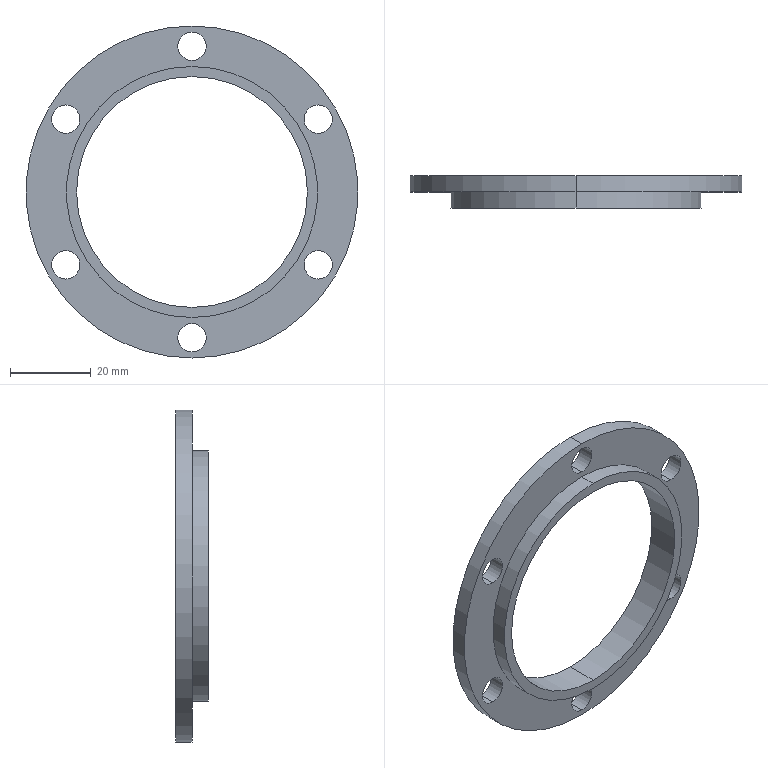Part | SolidWorks | features HoleWzd 2, ICE 1, Revolution 1 | 1 solid | 21 faces | box 82 x 8 x 82 mm | volume 11863 mm3 | cylinder 18 | plane 3 | commonest cylinder face diameters 7 x12 57 x2 62 x2 82 x2
STEP:
#1=CARTESIAN_POINT('',(-1069.592,74.472,129.));
#2=VERTEX_POINT('',#1);
#3=CARTESIAN_POINT('',(-1069.592,74.472,122.));
#4=VERTEX_POINT('',#3);
#5=CARTESIAN_POINT('',(-1069.592,74.472,125.5));
#6=DIRECTION('',(0.,-1.,0.));
#7=DIRECTION('',(0.,0.,-1.));
#8=AXIS2_PLACEMENT_3D('',#5,#6,#7);
#9=CIRCLE('',#8,3.5);
#10=EDGE_CURVE('',#2,#4,#9,.T.);
#11=ORIENTED_EDGE('',*,*,#10,.F.);
#12=CARTESIAN_POINT('',(-1069.592,70.472,129.));
#13=VERTEX_POINT('',#12);
#14=CARTESIAN_POINT('',(-1069.592,70.472,129.));
#15=DIRECTION('',(0.,-1.,0.));
#16=VECTOR('',#15,1000.);
#17=LINE('',#14,#16);
#18=EDGE_CURVE('',#2,#13,#17,.T.);
#19=ORIENTED_EDGE('',*,*,#18,.T.);
#20=CARTESIAN_POINT('',(-1069.592,70.472,122.));
#21=VERTEX_POINT('',#20);
#22=CARTESIAN_POINT('',(-1069.592,70.472,125.5));
#23=DIRECTION('',(0.,-1.,0.));
#24=DIRECTION('',(0.,0.,-1.));
#25=AXIS2_PLACEMENT_3D('',#22,#23,#24);
#26=CIRCLE('',#25,3.5);
#27=EDGE_CURVE('',#13,#21,#26,.T.);
#28=ORIENTED_EDGE('',*,*,#27,.T.);
#29=CARTESIAN_POINT('',(-1069.592,70.472,122.));
#30=DIRECTION('',(0.,-1.,0.));
#31=VECTOR('',#30,1000.);
#32=LINE('',#29,#31);
#33=EDGE_CURVE('',#4,#21,#32,.T.);
#34=ORIENTED_EDGE('',*,*,#33,.F.);
#35=EDGE_LOOP('',(#11,#19,#28,#34));
#36=FACE_OUTER_BOUND('',#35,.T.);
#37=CARTESIAN_POINT('',(-1069.592,70.472,125.5));
#38=DIRECTION('',(0.,-1.,0.));
#39=DIRECTION('',(0.,0.,-1.));
#40=AXIS2_PLACEMENT_3D('',#37,#38,#39);
#41=CYLINDRICAL_SURFACE('',#40,3.5);
#42=ADVANCED_FACE('',(#36),#41,.F.);
#43=CARTESIAN_POINT('',(-1100.769,74.472,111.));
#44=VERTEX_POINT('',#43);
#45=CARTESIAN_POINT('',(-1100.769,74.472,104.));
#46=VERTEX_POINT('',#45);
#47=CARTESIAN_POINT('',(-1100.769,74.472,107.5));
#48=DIRECTION('',(0.,-1.,0.));
#49=DIRECTION('',(0.,0.,-1.));
#50=AXIS2_PLACEMENT_3D('',#47,#48,#49);
#51=CIRCLE('',#50,3.5);
#52=EDGE_CURVE('',#44,#46,#51,.T.);
#53=ORIENTED_EDGE('',*,*,#52,.F.);
#54=CARTESIAN_POINT('',(-1100.769,70.472,111.));
#55=VERTEX_POINT('',#54);
#56=CARTESIAN_POINT('',(-1100.769,70.472,111.));
#57=DIRECTION('',(0.,-1.,0.));
#58=VECTOR('',#57,1000.);
#59=LINE('',#56,#58);
#60=EDGE_CURVE('',#44,#55,#59,.T.);
#61=ORIENTED_EDGE('',*,*,#60,.T.);
#62=CARTESIAN_POINT('',(-1100.769,70.472,104.));
#63=VERTEX_POINT('',#62);
#64=CARTESIAN_POINT('',(-1100.769,70.472,107.5));
#65=DIRECTION('',(0.,-1.,0.));
#66=DIRECTION('',(0.,0.,-1.));
#67=AXIS2_PLACEMENT_3D('',#64,#65,#66);
#68=CIRCLE('',#67,3.5);
#69=EDGE_CURVE('',#55,#63,#68,.T.);
#70=ORIENTED_EDGE('',*,*,#69,.T.);
#71=CARTESIAN_POINT('',(-1100.769,70.472,104.));
#72=DIRECTION('',(0.,-1.,0.));
#73=VECTOR('',#72,1000.);
#74=LINE('',#71,#73);
#75=EDGE_CURVE('',#46,#63,#74,.T.);
#76=ORIENTED_EDGE('',*,*,#75,.F.);
#77=EDGE_LOOP('',(#53,#61,#70,#76));
#78=FACE_OUTER_BOUND('',#77,.T.);
#79=CARTESIAN_POINT('',(-1100.769,70.472,107.5));
#80=DIRECTION('',(0.,-1.,0.));
#81=DIRECTION('',(0.,0.,-1.));
#82=AXIS2_PLACEMENT_3D('',#79,#80,#81);
#83=CYLINDRICAL_SURFACE('',#82,3.5);
#84=ADVANCED_FACE('',(#78),#83,.F.);
#85=CARTESIAN_POINT('',(-1100.769,74.472,75.));
#86=VERTEX_POINT('',#85);
#87=CARTESIAN_POINT('',(-1100.769,74.472,68.));
#88=VERTEX_POINT('',#87);
#89=CARTESIAN_POINT('',(-1100.769,74.472,71.5));
#90=DIRECTION('',(0.,-1.,0.));
#91=DIRECTION('',(0.,0.,-1.));
#92=AXIS2_PLACEMENT_3D('',#89,#90,#91);
#93=CIRCLE('',#92,3.5);
#94=EDGE_CURVE('',#86,#88,#93,.T.);
#95=ORIENTED_EDGE('',*,*,#94,.F.);
#96=CARTESIAN_POINT('',(-1100.769,70.472,75.));
#97=VERTEX_POINT('',#96);
#98=CARTESIAN_POINT('',(-1100.769,70.472,75.));
#99=DIRECTION('',(0.,-1.,0.));
#100=VECTOR('',#99,1000.);
#101=LINE('',#98,#100);
#102=EDGE_CURVE('',#86,#97,#101,.T.);
#103=ORIENTED_EDGE('',*,*,#102,.T.);
#104=CARTESIAN_POINT('',(-1100.769,70.472,68.));
#105=VERTEX_POINT('',#104);
#106=CARTESIAN_POINT('',(-1100.769,70.472,71.5));
#107=DIRECTION('',(0.,-1.,0.));
#108=DIRECTION('',(0.,0.,-1.));
#109=AXIS2_PLACEMENT_3D('',#106,#107,#108);
#110=CIRCLE('',#109,3.5);
#111=EDGE_CURVE('',#97,#105,#110,.T.);
#112=ORIENTED_EDGE('',*,*,#111,.T.);
#113=CARTESIAN_POINT('',(-1100.769,70.472,68.));
#114=DIRECTION('',(0.,-1.,0.));
#115=VECTOR('',#114,1000.);
#116=LINE('',#113,#115);
#117=EDGE_CURVE('',#88,#105,#116,.T.);
#118=ORIENTED_EDGE('',*,*,#117,.F.);
#119=EDGE_LOOP('',(#95,#103,#112,#118));
#120=FACE_OUTER_BOUND('',#119,.T.);
#121=CARTESIAN_POINT('',(-1100.769,70.472,71.5));
#122=DIRECTION('',(0.,-1.,0.));
#123=DIRECTION('',(0.,0.,-1.));
#124=AXIS2_PLACEMENT_3D('',#121,#122,#123);
#125=CYLINDRICAL_SURFACE('',#124,3.5);
#126=ADVANCED_FACE('',(#120),#125,.F.);
#127=CARTESIAN_POINT('',(-1069.592,74.472,57.));
#128=VERTEX_POINT('',#127);
#129=CARTESIAN_POINT('',(-1069.592,74.472,50.));
#130=VERTEX_POINT('',#129);
#131=CARTESIAN_POINT('',(-1069.592,74.472,53.5));
#132=DIRECTION('',(0.,-1.,0.));
#133=DIRECTION('',(0.,0.,-1.));
#134=AXIS2_PLACEMENT_3D('',#131,#132,#133);
#135=CIRCLE('',#134,3.5);
#136=EDGE_CURVE('',#128,#130,#135,.T.);
#137=ORIENTED_EDGE('',*,*,#136,.F.);
#138=CARTESIAN_POINT('',(-1069.592,70.472,57.));
#139=VERTEX_POINT('',#138);
#140=CARTESIAN_POINT('',(-1069.592,70.472,57.));
#141=DIRECTION('',(0.,-1.,0.));
#142=VECTOR('',#141,1000.);
#143=LINE('',#140,#142);
#144=EDGE_CURVE('',#128,#139,#143,.T.);
#145=ORIENTED_EDGE('',*,*,#144,.T.);
#146=CARTESIAN_POINT('',(-1069.592,70.472,50.));
#147=VERTEX_POINT('',#146);
#148=CARTESIAN_POINT('',(-1069.592,70.472,53.5));
#149=DIRECTION('',(0.,-1.,0.));
#150=DIRECTION('',(0.,0.,-1.));
#151=AXIS2_PLACEMENT_3D('',#148,#149,#150);
#152=CIRCLE('',#151,3.5);
#153=EDGE_CURVE('',#139,#147,#152,.T.);
#154=ORIENTED_EDGE('',*,*,#153,.T.);
#155=CARTESIAN_POINT('',(-1069.592,70.472,50.));
#156=DIRECTION('',(0.,-1.,0.));
#157=VECTOR('',#156,1000.);
#158=LINE('',#155,#157);
#159=EDGE_CURVE('',#130,#147,#158,.T.);
#160=ORIENTED_EDGE('',*,*,#159,.F.);
#161=EDGE_LOOP('',(#137,#145,#154,#160));
#162=FACE_OUTER_BOUND('',#161,.T.);
#163=CARTESIAN_POINT('',(-1069.592,70.472,53.5));
#164=DIRECTION('',(0.,-1.,0.));
#165=DIRECTION('',(0.,0.,-1.));
#166=AXIS2_PLACEMENT_3D('',#163,#164,#165);
#167=CYLINDRICAL_SURFACE('',#166,3.5);
#168=ADVANCED_FACE('',(#162),#167,.F.);
#169=CARTESIAN_POINT('',(-1038.415,74.472,75.));
#170=VERTEX_POINT('',#169);
#171=CARTESIAN_POINT('',(-1038.415,74.472,68.));
#172=VERTEX_POINT('',#171);
#173=CARTESIAN_POINT('',(-1038.415,74.472,71.5));
#174=DIRECTION('',(0.,-1.,0.));
#175=DIRECTION('',(0.,0.,-1.));
#176=AXIS2_PLACEMENT_3D('',#173,#174,#175);
#177=CIRCLE('',#176,3.5);
#178=EDGE_CURVE('',#170,#172,#177,.T.);
#179=ORIENTED_EDGE('',*,*,#178,.F.);
#180=CARTESIAN_POINT('',(-1038.415,70.472,75.));
#181=VERTEX_POINT('',#180);
#182=CARTESIAN_POINT('',(-1038.415,70.472,75.));
#183=DIRECTION('',(0.,-1.,0.));
#184=VECTOR('',#183,1000.);
#185=LINE('',#182,#184);
#186=EDGE_CURVE('',#170,#181,#185,.T.);
#187=ORIENTED_EDGE('',*,*,#186,.T.);
#188=CARTESIAN_POINT('',(-1038.415,70.472,68.));
#189=VERTEX_POINT('',#188);
#190=CARTESIAN_POINT('',(-1038.415,70.472,71.5));
#191=DIRECTION('',(0.,-1.,0.));
#192=DIRECTION('',(0.,0.,-1.));
#193=AXIS2_PLACEMENT_3D('',#190,#191,#192);
#194=CIRCLE('',#193,3.5);
#195=EDGE_CURVE('',#181,#189,#194,.T.);
#196=ORIENTED_EDGE('',*,*,#195,.T.);
#197=CARTESIAN_POINT('',(-1038.415,70.472,68.));
#198=DIRECTION('',(0.,-1.,0.));
#199=VECTOR('',#198,1000.);
#200=LINE('',#197,#199);
#201=EDGE_CURVE('',#172,#189,#200,.T.);
#202=ORIENTED_EDGE('',*,*,#201,.F.);
#203=EDGE_LOOP('',(#179,#187,#196,#202));
#204=FACE_OUTER_BOUND('',#203,.T.);
#205=CARTESIAN_POINT('',(-1038.415,70.472,71.5));
#206=DIRECTION('',(0.,-1.,0.));
#207=DIRECTION('',(0.,0.,-1.));
#208=AXIS2_PLACEMENT_3D('',#205,#206,#207);
#209=CYLINDRICAL_SURFACE('',#208,3.5);
#210=ADVANCED_FACE('',(#204),#209,.F.);
#211=CARTESIAN_POINT('',(-1038.415,74.472,111.));
#212=VERTEX_POINT('',#211);
#213=CARTESIAN_POINT('',(-1038.415,74.472,104.));
#214=VERTEX_POINT('',#213);
#215=CARTESIAN_POINT('',(-1038.415,74.472,107.5));
#216=DIRECTION('',(0.,-1.,0.));
#217=DIRECTION('',(0.,0.,-1.));
#218=AXIS2_PLACEMENT_3D('',#215,#216,#217);
#219=CIRCLE('',#218,3.5);
#220=EDGE_CURVE('',#212,#214,#219,.T.);
#221=ORIENTED_EDGE('',*,*,#220,.F.);
#222=CARTESIAN_POINT('',(-1038.415,70.472,111.));
#223=VERTEX_POINT('',#222);
#224=CARTESIAN_POINT('',(-1038.415,70.472,111.));
#225=DIRECTION('',(0.,-1.,0.));
#226=VECTOR('',#225,1000.);
#227=LINE('',#224,#226);
#228=EDGE_CURVE('',#212,#223,#227,.T.);
#229=ORIENTED_EDGE('',*,*,#228,.T.);
#230=CARTESIAN_POINT('',(-1038.415,70.472,104.));
#231=VERTEX_POINT('',#230);
#232=CARTESIAN_POINT('',(-1038.415,70.472,107.5));
#233=DIRECTION('',(0.,-1.,0.));
#234=DIRECTION('',(0.,0.,-1.));
#235=AXIS2_PLACEMENT_3D('',#232,#233,#234);
#236=CIRCLE('',#235,3.5);
#237=EDGE_CURVE('',#223,#231,#236,.T.);
#238=ORIENTED_EDGE('',*,*,#237,.T.);
#239=CARTESIAN_POINT('',(-1038.415,70.472,104.));
#240=DIRECTION('',(0.,-1.,0.));
#241=VECTOR('',#240,1000.);
#242=LINE('',#239,#241);
#243=EDGE_CURVE('',#214,#231,#242,.T.);
#244=ORIENTED_EDGE('',*,*,#243,.F.);
#245=EDGE_LOOP('',(#221,#229,#238,#244));
#246=FACE_OUTER_BOUND('',#245,.T.);
#247=CARTESIAN_POINT('',(-1038.415,70.472,107.5));
#248=DIRECTION('',(0.,-1.,0.));
#249=DIRECTION('',(0.,0.,-1.));
#250=AXIS2_PLACEMENT_3D('',#247,#248,#249);
#251=CYLINDRICAL_SURFACE('',#250,3.5);
#252=ADVANCED_FACE('',(#246),#251,.F.);
#253=CARTESIAN_POINT('',(-1069.592,74.472,118.));
#254=VERTEX_POINT('',#253);
#255=CARTESIAN_POINT('',(-1069.592,74.472,61.));
#256=VERTEX_POINT('',#255);
#257=CARTESIAN_POINT('',(-1069.592,74.472,89.5));
#258=DIRECTION('',(0.,-1.,0.));
#259=DIRECTION('',(0.,0.,-1.));
#260=AXIS2_PLACEMENT_3D('',#257,#258,#259);
#261=CIRCLE('',#260,28.5);
#262=EDGE_CURVE('',#254,#256,#261,.T.);
#263=ORIENTED_EDGE('',*,*,#262,.F.);
#264=CARTESIAN_POINT('',(-1069.592,66.472,118.));
#265=VERTEX_POINT('',#264);
#266=CARTESIAN_POINT('',(-1069.592,66.472,118.));
#267=DIRECTION('',(0.,-1.,0.));
#268=VECTOR('',#267,1000.);
#269=LINE('',#266,#268);
#270=EDGE_CURVE('',#254,#265,#269,.T.);
#271=ORIENTED_EDGE('',*,*,#270,.T.);
#272=CARTESIAN_POINT('',(-1069.592,66.472,61.));
#273=VERTEX_POINT('',#272);
#274=CARTESIAN_POINT('',(-1069.592,66.472,89.5));
#275=DIRECTION('',(0.,-1.,0.));
#276=DIRECTION('',(0.,0.,-1.));
#277=AXIS2_PLACEMENT_3D('',#274,#275,#276);
#278=CIRCLE('',#277,28.5);
#279=EDGE_CURVE('',#265,#273,#278,.T.);
#280=ORIENTED_EDGE('',*,*,#279,.T.);
#281=CARTESIAN_POINT('',(-1069.592,66.472,61.));
#282=DIRECTION('',(0.,-1.,0.));
#283=VECTOR('',#282,1000.);
#284=LINE('',#281,#283);
#285=EDGE_CURVE('',#256,#273,#284,.T.);
#286=ORIENTED_EDGE('',*,*,#285,.F.);
#287=EDGE_LOOP('',(#263,#271,#280,#286));
#288=FACE_OUTER_BOUND('',#287,.T.);
#289=CARTESIAN_POINT('',(-1069.592,66.472,89.5));
#290=DIRECTION('',(0.,-1.,0.));
#291=DIRECTION('',(0.,0.,-1.));
#292=AXIS2_PLACEMENT_3D('',#289,#290,#291);
#293=CYLINDRICAL_SURFACE('',#292,28.5);
#294=ADVANCED_FACE('',(#288),#293,.F.);
#295=CARTESIAN_POINT('',(-1069.592,66.472,58.5));
#296=VERTEX_POINT('',#295);
#297=CARTESIAN_POINT('',(-1069.592,66.472,120.5));
#298=VERTEX_POINT('',#297);
#299=CARTESIAN_POINT('',(-1069.592,66.472,89.5));
#300=DIRECTION('',(0.,-1.,0.));
#301=DIRECTION('',(0.,0.,-1.));
#302=AXIS2_PLACEMENT_3D('',#299,#300,#301);
#303=CIRCLE('',#302,31.);
#304=EDGE_CURVE('',#296,#298,#303,.T.);
#305=ORIENTED_EDGE('',*,*,#304,.F.);
#306=CARTESIAN_POINT('',(-1069.592,70.472,58.5));
#307=VERTEX_POINT('',#306);
#308=CARTESIAN_POINT('',(-1069.592,66.472,58.5));
#309=DIRECTION('',(0.,1.,0.));
#310=VECTOR('',#309,1000.);
#311=LINE('',#308,#310);
#312=EDGE_CURVE('',#296,#307,#311,.T.);
#313=ORIENTED_EDGE('',*,*,#312,.T.);
#314=CARTESIAN_POINT('',(-1069.592,70.472,120.5));
#315=VERTEX_POINT('',#314);
#316=CARTESIAN_POINT('',(-1069.592,70.472,89.5));
#317=DIRECTION('',(0.,-1.,0.));
#318=DIRECTION('',(0.,0.,-1.));
#319=AXIS2_PLACEMENT_3D('',#316,#317,#318);
#320=CIRCLE('',#319,31.);
#321=EDGE_CURVE('',#307,#315,#320,.T.);
#322=ORIENTED_EDGE('',*,*,#321,.T.);
#323=CARTESIAN_POINT('',(-1069.592,66.472,120.5));
#324=DIRECTION('',(0.,1.,0.));
#325=VECTOR('',#324,1000.);
#326=LINE('',#323,#325);
#327=EDGE_CURVE('',#298,#315,#326,.T.);
#328=ORIENTED_EDGE('',*,*,#327,.F.);
#329=EDGE_LOOP('',(#305,#313,#322,#328));
#330=FACE_OUTER_BOUND('',#329,.T.);
#331=CARTESIAN_POINT('',(-1069.592,66.472,89.5));
#332=DIRECTION('',(0.,1.,0.));
#333=DIRECTION('',(0.,0.,1.));
#334=AXIS2_PLACEMENT_3D('',#331,#332,#333);
#335=CYLINDRICAL_SURFACE('',#334,31.);
#336=ADVANCED_FACE('',(#330),#335,.T.);
#337=CARTESIAN_POINT('',(-1069.592,74.472,48.5));
#338=VERTEX_POINT('',#337);
#339=CARTESIAN_POINT('',(-1069.592,74.472,130.5));
#340=VERTEX_POINT('',#339);
#341=CARTESIAN_POINT('',(-1069.592,74.472,89.5));
#342=DIRECTION('',(0.,-1.,0.));
#343=DIRECTION('',(0.,0.,-1.));
#344=AXIS2_PLACEMENT_3D('',#341,#342,#343);
#345=CIRCLE('',#344,41.);
#346=EDGE_CURVE('',#338,#340,#345,.T.);
#347=ORIENTED_EDGE('',*,*,#346,.T.);
#348=CARTESIAN_POINT('',(-1069.592,70.472,130.5));
#349=VERTEX_POINT('',#348);
#350=CARTESIAN_POINT('',(-1069.592,74.472,130.5));
#351=DIRECTION('',(0.,-1.,0.));
#352=VECTOR('',#351,1000.);
#353=LINE('',#350,#352);
#354=EDGE_CURVE('',#340,#349,#353,.T.);
#355=ORIENTED_EDGE('',*,*,#354,.T.);
#356=CARTESIAN_POINT('',(-1069.592,70.472,48.5));
#357=VERTEX_POINT('',#356);
#358=CARTESIAN_POINT('',(-1069.592,70.472,89.5));
#359=DIRECTION('',(0.,-1.,0.));
#360=DIRECTION('',(0.,0.,-1.));
#361=AXIS2_PLACEMENT_3D('',#358,#359,#360);
#362=CIRCLE('',#361,41.);
#363=EDGE_CURVE('',#357,#349,#362,.T.);
#364=ORIENTED_EDGE('',*,*,#363,.F.);
#365=CARTESIAN_POINT('',(-1069.592,74.472,48.5));
#366=DIRECTION('',(0.,-1.,0.));
#367=VECTOR('',#366,1000.);
#368=LINE('',#365,#367);
#369=EDGE_CURVE('',#338,#357,#368,.T.);
#370=ORIENTED_EDGE('',*,*,#369,.F.);
#371=EDGE_LOOP('',(#347,#355,#364,#370));
#372=FACE_OUTER_BOUND('',#371,.T.);
#373=CARTESIAN_POINT('',(-1069.592,74.472,89.5));
#374=DIRECTION('',(0.,-1.,0.));
#375=DIRECTION('',(0.,0.,-1.));
#376=AXIS2_PLACEMENT_3D('',#373,#374,#375);
#377=CYLINDRICAL_SURFACE('',#376,41.);
#378=ADVANCED_FACE('',(#372),#377,.T.);
#379=ORIENTED_EDGE('',*,*,#354,.F.);
#380=CARTESIAN_POINT('',(-1069.592,74.472,89.5));
#381=DIRECTION('',(0.,-1.,0.));
#382=DIRECTION('',(0.,0.,-1.));
#383=AXIS2_PLACEMENT_3D('',#380,#381,#382);
#384=CIRCLE('',#383,41.);
#385=EDGE_CURVE('',#340,#338,#384,.T.);
#386=ORIENTED_EDGE('',*,*,#385,.T.);
#387=ORIENTED_EDGE('',*,*,#369,.T.);
#388=CARTESIAN_POINT('',(-1069.592,70.472,89.5));
#389=DIRECTION('',(0.,-1.,0.));
#390=DIRECTION('',(0.,0.,-1.));
#391=AXIS2_PLACEMENT_3D('',#388,#389,#390);
#392=CIRCLE('',#391,41.);
#393=EDGE_CURVE('',#349,#357,#392,.T.);
#394=ORIENTED_EDGE('',*,*,#393,.F.);
#395=EDGE_LOOP('',(#379,#386,#387,#394));
#396=FACE_OUTER_BOUND('',#395,.T.);
#397=CARTESIAN_POINT('',(-1069.592,74.472,89.5));
#398=DIRECTION('',(0.,-1.,0.));
#399=DIRECTION('',(0.,0.,-1.));
#400=AXIS2_PLACEMENT_3D('',#397,#398,#399);
#401=CYLINDRICAL_SURFACE('',#400,41.);
#402=ADVANCED_FACE('',(#396),#401,.T.);
#403=CARTESIAN_POINT('',(-1069.592,74.472,125.5));
#404=DIRECTION('',(0.,-1.,0.));
#405=DIRECTION('',(0.,0.,-1.));
#406=AXIS2_PLACEMENT_3D('',#403,#404,#405);
#407=CIRCLE('',#406,3.5);
#408=EDGE_CURVE('',#4,#2,#407,.T.);
#409=ORIENTED_EDGE('',*,*,#408,.T.);
#410=ORIENTED_EDGE('',*,*,#10,.T.);
#411=EDGE_LOOP('',(#409,#410));
#412=FACE_BOUND('',#411,.T.);
#413=CARTESIAN_POINT('',(-1100.769,74.472,107.5));
#414=DIRECTION('',(0.,-1.,0.));
#415=DIRECTION('',(0.,0.,-1.));
#416=AXIS2_PLACEMENT_3D('',#413,#414,#415);
#417=CIRCLE('',#416,3.5);
#418=EDGE_CURVE('',#46,#44,#417,.T.);
#419=ORIENTED_EDGE('',*,*,#418,.T.);
#420=ORIENTED_EDGE('',*,*,#52,.T.);
#421=EDGE_LOOP('',(#419,#420));
#422=FACE_BOUND('',#421,.T.);
#423=CARTESIAN_POINT('',(-1100.769,74.472,71.5));
#424=DIRECTION('',(0.,-1.,0.));
#425=DIRECTION('',(0.,0.,-1.));
#426=AXIS2_PLACEMENT_3D('',#423,#424,#425);
#427=CIRCLE('',#426,3.5);
#428=EDGE_CURVE('',#88,#86,#427,.T.);
#429=ORIENTED_EDGE('',*,*,#428,.T.);
#430=ORIENTED_EDGE('',*,*,#94,.T.);
#431=EDGE_LOOP('',(#429,#430));
#432=FACE_BOUND('',#431,.T.);
#433=CARTESIAN_POINT('',(-1069.592,74.472,53.5));
#434=DIRECTION('',(0.,-1.,0.));
#435=DIRECTION('',(0.,0.,-1.));
#436=AXIS2_PLACEMENT_3D('',#433,#434,#435);
#437=CIRCLE('',#436,3.5);
#438=EDGE_CURVE('',#130,#128,#437,.T.);
#439=ORIENTED_EDGE('',*,*,#438,.T.);
#440=ORIENTED_EDGE('',*,*,#136,.T.);
#441=EDGE_LOOP('',(#439,#440));
#442=FACE_BOUND('',#441,.T.);
#443=CARTESIAN_POINT('',(-1038.415,74.472,71.5));
#444=DIRECTION('',(0.,-1.,0.));
#445=DIRECTION('',(0.,0.,-1.));
#446=AXIS2_PLACEMENT_3D('',#443,#444,#445);
#447=CIRCLE('',#446,3.5);
#448=EDGE_CURVE('',#172,#170,#447,.T.);
#449=ORIENTED_EDGE('',*,*,#448,.T.);
#450=ORIENTED_EDGE('',*,*,#178,.T.);
#451=EDGE_LOOP('',(#449,#450));
#452=FACE_BOUND('',#451,.T.);
#453=CARTESIAN_POINT('',(-1038.415,74.472,107.5));
#454=DIRECTION('',(0.,-1.,0.));
#455=DIRECTION('',(0.,0.,-1.));
#456=AXIS2_PLACEMENT_3D('',#453,#454,#455);
#457=CIRCLE('',#456,3.5);
#458=EDGE_CURVE('',#214,#212,#457,.T.);
#459=ORIENTED_EDGE('',*,*,#458,.T.);
#460=ORIENTED_EDGE('',*,*,#220,.T.);
#461=EDGE_LOOP('',(#459,#460));
#462=FACE_BOUND('',#461,.T.);
#463=CARTESIAN_POINT('',(-1069.592,74.472,89.5));
#464=DIRECTION('',(0.,-1.,0.));
#465=DIRECTION('',(0.,0.,-1.));
#466=AXIS2_PLACEMENT_3D('',#463,#464,#465);
#467=CIRCLE('',#466,28.5);
#468=EDGE_CURVE('',#256,#254,#467,.T.);
#469=ORIENTED_EDGE('',*,*,#468,.T.);
#470=ORIENTED_EDGE('',*,*,#262,.T.);
#471=EDGE_LOOP('',(#469,#470));
#472=FACE_BOUND('',#471,.T.);
#473=ORIENTED_EDGE('',*,*,#346,.F.);
#474=ORIENTED_EDGE('',*,*,#385,.F.);
#475=EDGE_LOOP('',(#473,#474));
#476=FACE_OUTER_BOUND('',#475,.T.);
#477=CARTESIAN_POINT('',(-1028.592,74.472,89.5));
#478=DIRECTION('',(0.,1.,0.));
#479=DIRECTION('',(0.,0.,1.));
#480=AXIS2_PLACEMENT_3D('',#477,#478,#479);
#481=PLANE('',#480);
#482=ADVANCED_FACE('',(#412,#422,#432,#442,#452,#462,#472,#476),#481,.T.);
#483=CARTESIAN_POINT('',(-1069.592,70.472,125.5));
#484=DIRECTION('',(0.,-1.,0.));
#485=DIRECTION('',(0.,0.,-1.));
#486=AXIS2_PLACEMENT_3D('',#483,#484,#485);
#487=CIRCLE('',#486,3.5);
#488=EDGE_CURVE('',#21,#13,#487,.T.);
#489=ORIENTED_EDGE('',*,*,#488,.F.);
#490=ORIENTED_EDGE('',*,*,#27,.F.);
#491=EDGE_LOOP('',(#489,#490));
#492=FACE_BOUND('',#491,.T.);
#493=CARTESIAN_POINT('',(-1100.769,70.472,107.5));
#494=DIRECTION('',(0.,-1.,0.));
#495=DIRECTION('',(0.,0.,-1.));
#496=AXIS2_PLACEMENT_3D('',#493,#494,#495);
#497=CIRCLE('',#496,3.5);
#498=EDGE_CURVE('',#63,#55,#497,.T.);
#499=ORIENTED_EDGE('',*,*,#498,.F.);
#500=ORIENTED_EDGE('',*,*,#69,.F.);
#501=EDGE_LOOP('',(#499,#500));
#502=FACE_BOUND('',#501,.T.);
#503=CARTESIAN_POINT('',(-1100.769,70.472,71.5));
#504=DIRECTION('',(0.,-1.,0.));
#505=DIRECTION('',(0.,0.,-1.));
#506=AXIS2_PLACEMENT_3D('',#503,#504,#505);
#507=CIRCLE('',#506,3.5);
#508=EDGE_CURVE('',#105,#97,#507,.T.);
#509=ORIENTED_EDGE('',*,*,#508,.F.);
#510=ORIENTED_EDGE('',*,*,#111,.F.);
#511=EDGE_LOOP('',(#509,#510));
#512=FACE_BOUND('',#511,.T.);
#513=CARTESIAN_POINT('',(-1069.592,70.472,53.5));
#514=DIRECTION('',(0.,-1.,0.));
#515=DIRECTION('',(0.,0.,-1.));
#516=AXIS2_PLACEMENT_3D('',#513,#514,#515);
#517=CIRCLE('',#516,3.5);
#518=EDGE_CURVE('',#147,#139,#517,.T.);
#519=ORIENTED_EDGE('',*,*,#518,.F.);
#520=ORIENTED_EDGE('',*,*,#153,.F.);
#521=EDGE_LOOP('',(#519,#520));
#522=FACE_BOUND('',#521,.T.);
#523=CARTESIAN_POINT('',(-1038.415,70.472,71.5));
#524=DIRECTION('',(0.,-1.,0.));
#525=DIRECTION('',(0.,0.,-1.));
#526=AXIS2_PLACEMENT_3D('',#523,#524,#525);
#527=CIRCLE('',#526,3.5);
#528=EDGE_CURVE('',#189,#181,#527,.T.);
#529=ORIENTED_EDGE('',*,*,#528,.F.);
#530=ORIENTED_EDGE('',*,*,#195,.F.);
#531=EDGE_LOOP('',(#529,#530));
#532=FACE_BOUND('',#531,.T.);
#533=CARTESIAN_POINT('',(-1038.415,70.472,107.5));
#534=DIRECTION('',(0.,-1.,0.));
#535=DIRECTION('',(0.,0.,-1.));
#536=AXIS2_PLACEMENT_3D('',#533,#534,#535);
#537=CIRCLE('',#536,3.5);
#538=EDGE_CURVE('',#231,#223,#537,.T.);
#539=ORIENTED_EDGE('',*,*,#538,.F.);
#540=ORIENTED_EDGE('',*,*,#237,.F.);
#541=EDGE_LOOP('',(#539,#540));
#542=FACE_BOUND('',#541,.T.);
#543=CARTESIAN_POINT('',(-1069.592,70.472,89.5));
#544=DIRECTION('',(0.,-1.,0.));
#545=DIRECTION('',(0.,0.,-1.));
#546=AXIS2_PLACEMENT_3D('',#543,#544,#545);
#547=CIRCLE('',#546,31.);
#548=EDGE_CURVE('',#315,#307,#547,.T.);
#549=ORIENTED_EDGE('',*,*,#548,.F.);
#550=ORIENTED_EDGE('',*,*,#321,.F.);
#551=EDGE_LOOP('',(#549,#550));
#552=FACE_BOUND('',#551,.T.);
#553=ORIENTED_EDGE('',*,*,#363,.T.);
#554=ORIENTED_EDGE('',*,*,#393,.T.);
#555=EDGE_LOOP('',(#553,#554));
#556=FACE_OUTER_BOUND('',#555,.T.);
#557=CARTESIAN_POINT('',(-1069.592,70.472,89.5));
#558=DIRECTION('',(0.,-1.,0.));
#559=DIRECTION('',(0.,0.,-1.));
#560=AXIS2_PLACEMENT_3D('',#557,#558,#559);
#561=PLANE('',#560);
#562=ADVANCED_FACE('',(#492,#502,#512,#522,#532,#542,#552,#556),#561,.T.);
#563=ORIENTED_EDGE('',*,*,#312,.F.);
#564=CARTESIAN_POINT('',(-1069.592,66.472,89.5));
#565=DIRECTION('',(0.,-1.,0.));
#566=DIRECTION('',(0.,0.,-1.));
#567=AXIS2_PLACEMENT_3D('',#564,#565,#566);
#568=CIRCLE('',#567,31.);
#569=EDGE_CURVE('',#298,#296,#568,.T.);
#570=ORIENTED_EDGE('',*,*,#569,.F.);
#571=ORIENTED_EDGE('',*,*,#327,.T.);
#572=ORIENTED_EDGE('',*,*,#548,.T.);
#573=EDGE_LOOP('',(#563,#570,#571,#572));
#574=FACE_OUTER_BOUND('',#573,.T.);
#575=CARTESIAN_POINT('',(-1069.592,66.472,89.5));
#576=DIRECTION('',(0.,1.,0.));
#577=DIRECTION('',(0.,0.,1.));
#578=AXIS2_PLACEMENT_3D('',#575,#576,#577);
#579=CYLINDRICAL_SURFACE('',#578,31.);
#580=ADVANCED_FACE('',(#574),#579,.T.);
#581=CARTESIAN_POINT('',(-1069.592,66.472,89.5));
#582=DIRECTION('',(0.,-1.,0.));
#583=DIRECTION('',(0.,0.,-1.));
#584=AXIS2_PLACEMENT_3D('',#581,#582,#583);
#585=CIRCLE('',#584,28.5);
#586=EDGE_CURVE('',#273,#265,#585,.T.);
#587=ORIENTED_EDGE('',*,*,#586,.F.);
#588=ORIENTED_EDGE('',*,*,#279,.F.);
#589=EDGE_LOOP('',(#587,#588));
#590=FACE_BOUND('',#589,.T.);
#591=ORIENTED_EDGE('',*,*,#569,.T.);
#592=ORIENTED_EDGE('',*,*,#304,.T.);
#593=EDGE_LOOP('',(#591,#592));
#594=FACE_OUTER_BOUND('',#593,.T.);
#595=CARTESIAN_POINT('',(-1069.592,66.472,89.5));
#596=DIRECTION('',(0.,-1.,0.));
#597=DIRECTION('',(0.,0.,-1.));
#598=AXIS2_PLACEMENT_3D('',#595,#596,#597);
#599=PLANE('',#598);
#600=ADVANCED_FACE('',(#590,#594),#599,.T.);
#601=ORIENTED_EDGE('',*,*,#270,.F.);
#602=ORIENTED_EDGE('',*,*,#468,.F.);
#603=ORIENTED_EDGE('',*,*,#285,.T.);
#604=ORIENTED_EDGE('',*,*,#586,.T.);
#605=EDGE_LOOP('',(#601,#602,#603,#604));
#606=FACE_OUTER_BOUND('',#605,.T.);
#607=CARTESIAN_POINT('',(-1069.592,66.472,89.5));
#608=DIRECTION('',(0.,-1.,0.));
#609=DIRECTION('',(0.,0.,-1.));
#610=AXIS2_PLACEMENT_3D('',#607,#608,#609);
#611=CYLINDRICAL_SURFACE('',#610,28.5);
#612=ADVANCED_FACE('',(#606),#611,.F.);
#613=ORIENTED_EDGE('',*,*,#228,.F.);
#614=ORIENTED_EDGE('',*,*,#458,.F.);
#615=ORIENTED_EDGE('',*,*,#243,.T.);
#616=ORIENTED_EDGE('',*,*,#538,.T.);
#617=EDGE_LOOP('',(#613,#614,#615,#616));
#618=FACE_OUTER_BOUND('',#617,.T.);
#619=CARTESIAN_POINT('',(-1038.415,70.472,107.5));
#620=DIRECTION('',(0.,-1.,0.));
#621=DIRECTION('',(0.,0.,-1.));
#622=AXIS2_PLACEMENT_3D('',#619,#620,#621);
#623=CYLINDRICAL_SURFACE('',#622,3.5);
#624=ADVANCED_FACE('',(#618),#623,.F.);
#625=ORIENTED_EDGE('',*,*,#186,.F.);
#626=ORIENTED_EDGE('',*,*,#448,.F.);
#627=ORIENTED_EDGE('',*,*,#201,.T.);
#628=ORIENTED_EDGE('',*,*,#528,.T.);
#629=EDGE_LOOP('',(#625,#626,#627,#628));
#630=FACE_OUTER_BOUND('',#629,.T.);
#631=CARTESIAN_POINT('',(-1038.415,70.472,71.5));
#632=DIRECTION('',(0.,-1.,0.));
#633=DIRECTION('',(0.,0.,-1.));
#634=AXIS2_PLACEMENT_3D('',#631,#632,#633);
#635=CYLINDRICAL_SURFACE('',#634,3.5);
#636=ADVANCED_FACE('',(#630),#635,.F.);
#637=ORIENTED_EDGE('',*,*,#144,.F.);
#638=ORIENTED_EDGE('',*,*,#438,.F.);
#639=ORIENTED_EDGE('',*,*,#159,.T.);
#640=ORIENTED_EDGE('',*,*,#518,.T.);
#641=EDGE_LOOP('',(#637,#638,#639,#640));
#642=FACE_OUTER_BOUND('',#641,.T.);
#643=CARTESIAN_POINT('',(-1069.592,70.472,53.5));
#644=DIRECTION('',(0.,-1.,0.));
#645=DIRECTION('',(0.,0.,-1.));
#646=AXIS2_PLACEMENT_3D('',#643,#644,#645);
#647=CYLINDRICAL_SURFACE('',#646,3.5);
#648=ADVANCED_FACE('',(#642),#647,.F.);
#649=ORIENTED_EDGE('',*,*,#102,.F.);
#650=ORIENTED_EDGE('',*,*,#428,.F.);
#651=ORIENTED_EDGE('',*,*,#117,.T.);
#652=ORIENTED_EDGE('',*,*,#508,.T.);
#653=EDGE_LOOP('',(#649,#650,#651,#652));
#654=FACE_OUTER_BOUND('',#653,.T.);
#655=CARTESIAN_POINT('',(-1100.769,70.472,71.5));
#656=DIRECTION('',(0.,-1.,0.));
#657=DIRECTION('',(0.,0.,-1.));
#658=AXIS2_PLACEMENT_3D('',#655,#656,#657);
#659=CYLINDRICAL_SURFACE('',#658,3.5);
#660=ADVANCED_FACE('',(#654),#659,.F.);
#661=ORIENTED_EDGE('',*,*,#60,.F.);
#662=ORIENTED_EDGE('',*,*,#418,.F.);
#663=ORIENTED_EDGE('',*,*,#75,.T.);
#664=ORIENTED_EDGE('',*,*,#498,.T.);
#665=EDGE_LOOP('',(#661,#662,#663,#664));
#666=FACE_OUTER_BOUND('',#665,.T.);
#667=CARTESIAN_POINT('',(-1100.769,70.472,107.5));
#668=DIRECTION('',(0.,-1.,0.));
#669=DIRECTION('',(0.,0.,-1.));
#670=AXIS2_PLACEMENT_3D('',#667,#668,#669);
#671=CYLINDRICAL_SURFACE('',#670,3.5);
#672=ADVANCED_FACE('',(#666),#671,.F.);
#673=ORIENTED_EDGE('',*,*,#18,.F.);
#674=ORIENTED_EDGE('',*,*,#408,.F.);
#675=ORIENTED_EDGE('',*,*,#33,.T.);
#676=ORIENTED_EDGE('',*,*,#488,.T.);
#677=EDGE_LOOP('',(#673,#674,#675,#676));
#678=FACE_OUTER_BOUND('',#677,.T.);
#679=CARTESIAN_POINT('',(-1069.592,70.472,125.5));
#680=DIRECTION('',(0.,-1.,0.));
#681=DIRECTION('',(0.,0.,-1.));
#682=AXIS2_PLACEMENT_3D('',#679,#680,#681);
#683=CYLINDRICAL_SURFACE('',#682,3.5);
#684=ADVANCED_FACE('',(#678),#683,.F.);
#685=CLOSED_SHELL('',(#42,#84,#126,#168,#210,#252,#294,#336,#378,#402,#482,#562,#580,#600,#612,#624,#636,#648,#660,#672,#684));
#686=MANIFOLD_SOLID_BREP('',#685);
#687=CARTESIAN_POINT('',(0.,0.,0.));
#688=DIRECTION('',(0.,0.,1.));
#689=DIRECTION('',(1.,0.,0.));
#690=AXIS2_PLACEMENT_3D('',#687,#688,#689);
#691=(LENGTH_UNIT()NAMED_UNIT(*)SI_UNIT(.MILLI.,.METRE.));
#692=UNCERTAINTY_MEASURE_WITH_UNIT(LENGTH_MEASURE(0.00001),#691,'','');
#693=(NAMED_UNIT(*)PLANE_ANGLE_UNIT()SI_UNIT($,.RADIAN.));
#694=(NAMED_UNIT(*)SI_UNIT($,.STERADIAN.)SOLID_ANGLE_UNIT());
#695=(GEOMETRIC_REPRESENTATION_CONTEXT(3)GLOBAL_UNCERTAINTY_ASSIGNED_CONTEXT((#692))GLOBAL_UNIT_ASSIGNED_CONTEXT((#691,#693,#694))REPRESENTATION_CONTEXT('',''));
#696=ADVANCED_BREP_SHAPE_REPRESENTATION('',(#686,#690),#695);